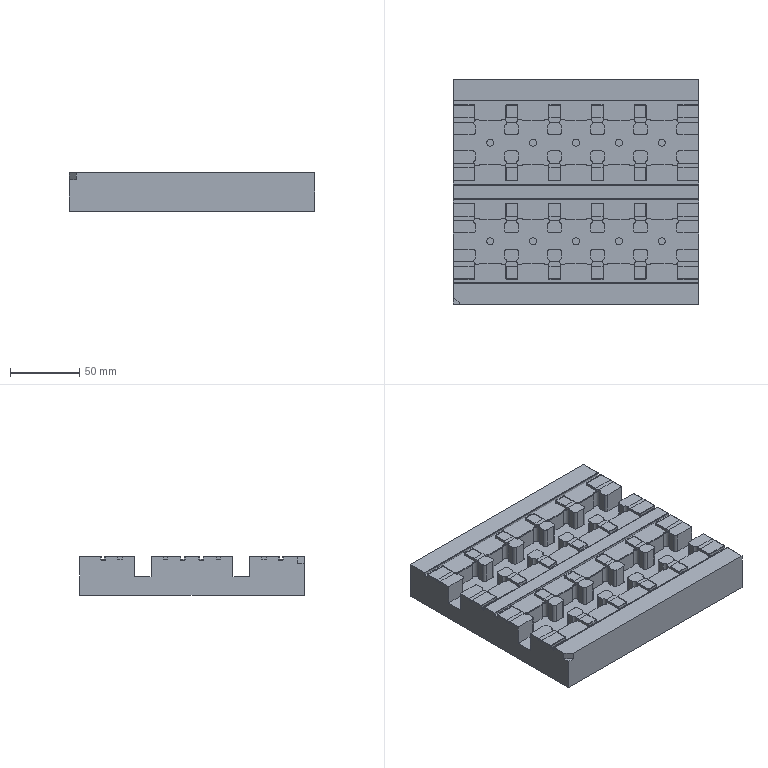NC program | NX | posted by the shop | part box 177 x 162 x 28 mm
Whole program:
%
O0001
(Machine time: 41.63 MIN)
(===Total Tool:4===)
(T2=D17R0.8FlyCutter D=17.  R=0.8  D-  H02 Z=1.    )
(T10=D10    D=10.  R=0.   D10 H10 Z=1.5   )
(T11=D10-J  D=10.  R=0.   D-  H11 Z=1.5   )
(T1=D6ChamferMill   D=6.   R=0.   D-  H01 Z=28.5  )
G80 G90 G17 G49 G40
G91 G28 Z0
M01
N1 T02 M06
(D17R0.8FlyCutter  D=17. R=0.8 H=02 ce=0.20 di=0.10)
(MAX_Z=45. MIN_Z=1. Time=26.17M)
T10
G00 G90 G54 X-109. Y78.971 M03 S2000
G43 H02 Z45.
M08
Z32.3
G01 Z30.3 F3000.
X-97.
X97.
Y68.441
X-97.
Y57.912
X97.
Y47.382
X-97.
Y36.853
X97.
Y26.324
X-97.
Y15.794
X97.
Y5.265
X-97.
Y-5.265
X97.
Y-15.794
X-97.
Y-26.324
X97.
Y-36.853
X-97.
Y-47.382
X97.
Y-57.912
X-97.
Y-68.441
X97.
Y-78.971
X-97.
X-109.
Z32.3
G00 Z33.5
Y78.971
Z32.1
G01 Z30.1
X-97.
X97.
Y68.441
X-97.
Y57.912
X97.
Y47.382
X-97.
Y36.853
X97.
Y26.324
X-97.
Y15.794
X97.
Y5.265
X-97.
Y-5.265
X97.
Y-15.794
X-97.
Y-26.324
X97.
Y-36.853
X-97.
Y-47.382
X97.
Y-57.912
X-97.
Y-68.441
X97.
Y-78.971
X-97.
X-109.
Z32.1
G00 Z45.
G00 G90 X97.2 Y-75.602 M03 S2000
Z45.
Z31.
G01 Y-81.723 Z30.679 F3000.
X96.795 Y-83.722 Z30.572
X95.937 Y-85.572 Z30.465
X94.673 Y-87.173 Z30.359
X93.072 Y-88.437 Z30.252
X91.222 Y-89.295 Z30.145
X89.223 Y-89.7 Z30.038
X88.5 Z30.
X-88.5 Z29.928
G02 X-97.2 Y-81. Z29.922 I0.0 J8.7
G01 Y81. Z29.856
G02 X-88.5 Y89.7 Z29.851 I8.7 J0.0
G01 X88.5 Z29.778
G02 X97.2 Y81. Z29.773 I0.0 J-8.7
G01 Y-81. Z29.707
G02 X88.5 Y-89.7 Z29.701 I-8.7 J0.0
G01 X-88.5 Z29.629
G02 X-97.2 Y-81. Z29.623 I0.0 J8.7
G01 Y81. Z29.557
G02 X-88.5 Y89.7 Z29.552 I8.7 J0.0
G01 X88.5 Z29.479
G02 X97.2 Y81. Z29.474 I0.0 J-8.7
G01 Y-81. Z29.408
G02 X88.5 Y-89.7 Z29.402 I-8.7 J0.0
G01 X-88.5 Z29.33
G02 X-97.2 Y-81. Z29.324 I0.0 J8.7
G01 Y81. Z29.258
G02 X-88.5 Y89.7 Z29.253 I8.7 J0.0
G01 X88.5 Z29.18
G02 X97.2 Y81. Z29.175 I0.0 J-8.7
G01 Y-81. Z29.109
G02 X88.5 Y-89.7 Z29.103 I-8.7 J0.0
G01 X-88.5 Z29.031
G02 X-97.2 Y-81. Z29.025 I0.0 J8.7
G01 Y81. Z28.959
G02 X-88.5 Y89.7 Z28.954 I8.7 J0.0
G01 X88.5 Z28.881
G02 X97.2 Y81. Z28.876 I0.0 J-8.7
G01 Y-81. Z28.81
G02 X88.5 Y-89.7 Z28.804 I-8.7 J0.0
G01 X-88.5 Z28.732
G02 X-97.2 Y-81. Z28.726 I0.0 J8.7
G01 Y81. Z28.66
G02 X-88.5 Y89.7 Z28.655 I8.7 J0.0
G01 X88.5 Z28.582
G02 X97.2 Y81. Z28.577 I0.0 J-8.7
G01 Y-81. Z28.511
G02 X88.5 Y-89.7 Z28.505 I-8.7 J0.0
G01 X-88.5 Z28.433
G02 X-97.2 Y-81. Z28.427 I0.0 J8.7
G01 Y81. Z28.361
G02 X-88.5 Y89.7 Z28.356 I8.7 J0.0
G01 X88.5 Z28.283
G02 X97.2 Y81. Z28.278 I0.0 J-8.7
G01 Y-81. Z28.212
G02 X88.5 Y-89.7 Z28.206 I-8.7 J0.0
G01 X-88.5 Z28.134
G02 X-97.2 Y-81. Z28.128 I0.0 J8.7
G01 Y81. Z28.062
G02 X-88.5 Y89.7 Z28.057 I8.7 J0.0
G01 X88.5 Z27.984
G02 X97.2 Y81. Z27.979 I0.0 J-8.7
G01 Y-81. Z27.913
G02 X88.5 Y-89.7 Z27.907 I-8.7 J0.0
G01 X-88.5 Z27.835
G02 X-97.2 Y-81. Z27.829 I0.0 J8.7
G01 Y81. Z27.763
G02 X-88.5 Y89.7 Z27.758 I8.7 J0.0
G01 X88.5 Z27.686
G02 X97.2 Y81. Z27.68 I0.0 J-8.7
G01 Y-81. Z27.614
G02 X88.5 Y-89.7 Z27.608 I-8.7 J0.0
G01 X-88.5 Z27.536
G02 X-97.2 Y-81. Z27.53 I0.0 J8.7
G01 Y81. Z27.464
G02 X-88.5 Y89.7 Z27.459 I8.7 J0.0
G01 X88.5 Z27.387
G02 X97.2 Y81. Z27.381 I0.0 J-8.7
G01 Y-81. Z27.315
G02 X88.5 Y-89.7 Z27.309 I-8.7 J0.0
G01 X-88.5 Z27.237
G02 X-97.2 Y-81. Z27.231 I0.0 J8.7
G01 Y81. Z27.165
G02 X-88.5 Y89.7 Z27.16 I8.7 J0.0
G01 X88.5 Z27.088
G02 X97.2 Y81. Z27.082 I0.0 J-8.7
G01 Y-81. Z27.016
G02 X88.5 Y-89.7 Z27.01 I-8.7 J0.0
G01 X-88.5 Z26.938
G02 X-97.2 Y-81. Z26.933 I0.0 J8.7
G01 Y81. Z26.866
G02 X-88.5 Y89.7 Z26.861 I8.7 J0.0
G01 X88.5 Z26.789
G02 X97.2 Y81. Z26.783 I0.0 J-8.7
G01 Y-81. Z26.717
G02 X88.5 Y-89.7 Z26.711 I-8.7 J0.0
G01 X-88.5 Z26.639
G02 X-97.2 Y-81. Z26.634 I0.0 J8.7
G01 Y81. Z26.567
G02 X-88.5 Y89.7 Z26.562 I8.7 J0.0
G01 X88.5 Z26.49
G02 X97.2 Y81. Z26.484 I0.0 J-8.7
G01 Y-81. Z26.418
G02 X88.5 Y-89.7 Z26.412 I-8.7 J0.0
G01 X-88.5 Z26.34
G02 X-97.2 Y-81. Z26.335 I0.0 J8.7
G01 Y81. Z26.268
G02 X-88.5 Y89.7 Z26.263 I8.7 J0.0
G01 X88.5 Z26.191
G02 X97.2 Y81. Z26.185 I0.0 J-8.7
G01 Y-81. Z26.119
G02 X88.5 Y-89.7 Z26.113 I-8.7 J0.0
G01 X-88.5 Z26.041
G02 X-97.2 Y-81. Z26.036 I0.0 J8.7
G01 Y81. Z25.969
G02 X-88.5 Y89.7 Z25.964 I8.7 J0.0
G01 X88.5 Z25.892
G02 X97.2 Y81. Z25.886 I0.0 J-8.7
G01 Y-81. Z25.82
G02 X88.5 Y-89.7 Z25.814 I-8.7 J0.0
G01 X-88.5 Z25.742
G02 X-97.2 Y-81. Z25.737 I0.0 J8.7
G01 Y81. Z25.671
G02 X-88.5 Y89.7 Z25.665 I8.7 J0.0
G01 X88.5 Z25.593
G02 X97.2 Y81. Z25.587 I0.0 J-8.7
G01 Y-81. Z25.521
G02 X88.5 Y-89.7 Z25.515 I-8.7 J0.0
G01 X-88.5 Z25.443
G02 X-97.2 Y-81. Z25.438 I0.0 J8.7
G01 Y81. Z25.372
G02 X-88.5 Y89.7 Z25.366 I8.7 J0.0
G01 X88.5 Z25.294
G02 X97.2 Y81. Z25.288 I0.0 J-8.7
G01 Y-81. Z25.222
G02 X88.5 Y-89.7 Z25.216 I-8.7 J0.0
G01 X-88.5 Z25.144
G02 X-97.2 Y-81. Z25.139 I0.0 J8.7
G01 Y81. Z25.073
G02 X-88.5 Y89.7 Z25.067 I8.7 J0.0
G01 X88.5 Z24.995
G02 X97.2 Y81. Z24.989 I0.0 J-8.7
G01 Y-81. Z24.923
G02 X88.5 Y-89.7 Z24.918 I-8.7 J0.0
G01 X-88.5 Z24.845
G02 X-97.2 Y-81. Z24.84 I0.0 J8.7
G01 Y81. Z24.774
G02 X-88.5 Y89.7 Z24.768 I8.7 J0.0
G01 X88.5 Z24.696
G02 X97.2 Y81. Z24.69 I0.0 J-8.7
G01 Y-81. Z24.624
G02 X88.5 Y-89.7 Z24.619 I-8.7 J0.0
G01 X-88.5 Z24.546
G02 X-97.2 Y-81. Z24.541 I0.0 J8.7
G01 Y81. Z24.475
G02 X-88.5 Y89.7 Z24.469 I8.7 J0.0
G01 X88.5 Z24.397
G02 X97.2 Y81. Z24.391 I0.0 J-8.7
G01 Y-81. Z24.325
G02 X88.5 Y-89.7 Z24.32 I-8.7 J0.0
G01 X-88.5 Z24.247
G02 X-97.2 Y-81. Z24.242 I0.0 J8.7
G01 Y81. Z24.176
G02 X-88.5 Y89.7 Z24.17 I8.7 J0.0
G01 X88.5 Z24.098
G02 X97.2 Y81. Z24.092 I0.0 J-8.7
G01 Y-81. Z24.026
G02 X88.5 Y-89.7 Z24.021 I-8.7 J0.0
G01 X-88.5 Z23.948
G02 X-97.2 Y-81. Z23.943 I0.0 J8.7
G01 Y81. Z23.877
G02 X-88.5 Y89.7 Z23.871 I8.7 J0.0
G01 X88.5 Z23.799
G02 X97.2 Y81. Z23.793 I0.0 J-8.7
G01 Y-81. Z23.727
G02 X88.5 Y-89.7 Z23.722 I-8.7 J0.0
G01 X-88.5 Z23.649
G02 X-97.2 Y-81. Z23.644 I0.0 J8.7
G01 Y81. Z23.578
G02 X-88.5 Y89.7 Z23.572 I8.7 J0.0
G01 X88.5 Z23.5
G02 X97.2 Y81. Z23.494 I0.0 J-8.7
G01 Y-81. Z23.428
G02 X88.5 Y-89.7 Z23.423 I-8.7 J0.0
G01 X-88.5 Z23.35
G02 X-97.2 Y-81. Z23.345 I0.0 J8.7
G01 Y81. Z23.279
G02 X-88.5 Y89.7 Z23.273 I8.7 J0.0
G01 X88.5 Z23.201
G02 X97.2 Y81. Z23.195 I0.0 J-8.7
G01 Y-81. Z23.129
G02 X88.5 Y-89.7 Z23.124 I-8.7 J0.0
G01 X-88.5 Z23.051
G02 X-97.2 Y-81. Z23.046 I0.0 J8.7
G01 Y81. Z22.98
G02 X-88.5 Y89.7 Z22.974 I8.7 J0.0
G01 X88.5 Z22.902
G02 X97.2 Y81. Z22.896 I0.0 J-8.7
G01 Y-81. Z22.83
G02 X88.5 Y-89.7 Z22.825 I-8.7 J0.0
G01 X-88.5 Z22.753
G02 X-97.2 Y-81. Z22.747 I0.0 J8.7
G01 Y81. Z22.681
G02 X-88.5 Y89.7 Z22.675 I8.7 J0.0
G01 X88.5 Z22.603
G02 X97.2 Y81. Z22.597 I0.0 J-8.7
G01 Y-81. Z22.531
G02 X88.5 Y-89.7 Z22.526 I-8.7 J0.0
G01 X-88.5 Z22.454
G02 X-97.2 Y-81. Z22.448 I0.0 J8.7
G01 Y81. Z22.382
G02 X-88.5 Y89.7 Z22.376 I8.7 J0.0
G01 X88.5 Z22.304
G02 X97.2 Y81. Z22.298 I0.0 J-8.7
G01 Y-81. Z22.232
G02 X88.5 Y-89.7 Z22.227 I-8.7 J0.0
G01 X-88.5 Z22.155
G02 X-97.2 Y-81. Z22.149 I0.0 J8.7
G01 Y81. Z22.083
G02 X-88.5 Y89.7 Z22.077 I8.7 J0.0
G01 X88.5 Z22.005
G02 X97.2 Y81. Z22. I0.0 J-8.7
G01 Y-81. Z21.933
G02 X88.5 Y-89.7 Z21.928 I-8.7 J0.0
G01 X-88.5 Z21.856
G02 X-97.2 Y-81. Z21.85 I0.0 J8.7
G01 Y81. Z21.784
G02 X-88.5 Y89.7 Z21.778 I8.7 J0.0
G01 X88.5 Z21.706
G02 X97.2 Y81. Z21.701 I0.0 J-8.7
G01 Y-81. Z21.634
G02 X88.5 Y-89.7 Z21.629 I-8.7 J0.0
G01 X-88.5 Z21.557
G02 X-97.2 Y-81. Z21.551 I0.0 J8.7
G01 Y81. Z21.485
G02 X-88.5 Y89.7 Z21.479 I8.7 J0.0
G01 X88.5 Z21.407
G02 X97.2 Y81. Z21.402 I0.0 J-8.7
G01 Y-81. Z21.335
G02 X88.5 Y-89.7 Z21.33 I-8.7 J0.0
G01 X-88.5 Z21.258
G02 X-97.2 Y-81. Z21.252 I0.0 J8.7
G01 Y81. Z21.186
G02 X-88.5 Y89.7 Z21.18 I8.7 J0.0
G01 X88.5 Z21.108
G02 X97.2 Y81. Z21.103 I0.0 J-8.7
G01 Y-81. Z21.037
G02 X88.5 Y-89.7 Z21.031 I-8.7 J0.0
G01 X-88.5 Z20.959
G02 X-97.2 Y-81. Z20.953 I0.0 J8.7
G01 Y81. Z20.887
G02 X-88.5 Y89.7 Z20.881 I8.7 J0.0
G01 X88.5 Z20.809
G02 X97.2 Y81. Z20.804 I0.0 J-8.7
G01 Y-81. Z20.738
G02 X88.5 Y-89.7 Z20.732 I-8.7 J0.0
G01 X-88.5 Z20.66
G02 X-97.2 Y-81. Z20.654 I0.0 J8.7
G01 Y81. Z20.588
G02 X-88.5 Y89.7 Z20.582 I8.7 J0.0
G01 X88.5 Z20.51
G02 X97.2 Y81. Z20.505 I0.0 J-8.7
G01 Y-81. Z20.439
G02 X88.5 Y-89.7 Z20.433 I-8.7 J0.0
G01 X-88.5 Z20.361
G02 X-97.2 Y-81. Z20.355 I0.0 J8.7
G01 Y81. Z20.289
G02 X-88.5 Y89.7 Z20.284 I8.7 J0.0
G01 X88.5 Z20.211
G02 X97.2 Y81. Z20.206 I0.0 J-8.7
G01 Y-81. Z20.14
G02 X88.5 Y-89.7 Z20.134 I-8.7 J0.0
G01 X-88.5 Z20.062
G02 X-97.2 Y-81. Z20.056 I0.0 J8.7
G01 Y81. Z19.99
G02 X-88.5 Y89.7 Z19.985 I8.7 J0.0
G01 X88.5 Z19.912
G02 X97.2 Y81. Z19.907 I0.0 J-8.7
G01 Y-81. Z19.841
G02 X88.5 Y-89.7 Z19.835 I-8.7 J0.0
G01 X-88.5 Z19.763
G02 X-97.2 Y-81. Z19.757 I0.0 J8.7
G01 Y81. Z19.691
G02 X-88.5 Y89.7 Z19.686 I8.7 J0.0
G01 X88.5 Z19.613
G02 X97.2 Y81. Z19.608 I0.0 J-8.7
G01 Y-81. Z19.542
G02 X88.5 Y-89.7 Z19.536 I-8.7 J0.0
G01 X-88.5 Z19.464
G02 X-97.2 Y-81. Z19.458 I0.0 J8.7
G01 Y81. Z19.392
G02 X-88.5 Y89.7 Z19.387 I8.7 J0.0
G01 X88.5 Z19.314
G02 X97.2 Y81. Z19.309 I0.0 J-8.7
G01 Y-81. Z19.243
G02 X88.5 Y-89.7 Z19.237 I-8.7 J0.0
G01 X-88.5 Z19.165
G02 X-97.2 Y-81. Z19.159 I0.0 J8.7
G01 Y81. Z19.093
G02 X-88.5 Y89.7 Z19.088 I8.7 J0.0
G01 X88.5 Z19.015
G02 X97.2 Y81. Z19.01 I0.0 J-8.7
G01 Y-81. Z18.944
G02 X88.5 Y-89.7 Z18.938 I-8.7 J0.0
G01 X-88.5 Z18.866
G02 X-97.2 Y-81. Z18.86 I0.0 J8.7
G01 Y81. Z18.794
G02 X-88.5 Y89.7 Z18.789 I8.7 J0.0
G01 X88.5 Z18.716
G02 X97.2 Y81. Z18.711 I0.0 J-8.7
G01 Y-81. Z18.645
G02 X88.5 Y-89.7 Z18.639 I-8.7 J0.0
G01 X-88.5 Z18.567
G02 X-97.2 Y-81. Z18.561 I0.0 J8.7
G01 Y81. Z18.495
G02 X-88.5 Y89.7 Z18.49 I8.7 J0.0
G01 X88.5 Z18.417
G02 X97.2 Y81. Z18.412 I0.0 J-8.7
G01 Y-81. Z18.346
G02 X88.5 Y-89.7 Z18.34 I-8.7 J0.0
G01 X-88.5 Z18.268
G02 X-97.2 Y-81. Z18.262 I0.0 J8.7
G01 Y81. Z18.196
G02 X-88.5 Y89.7 Z18.191 I8.7 J0.0
G01 X88.5 Z18.118
G02 X97.2 Y81. Z18.113 I0.0 J-8.7
G01 Y-81. Z18.047
G02 X88.5 Y-89.7 Z18.041 I-8.7 J0.0
G01 X-88.5 Z17.969
G02 X-97.2 Y-81. Z17.963 I0.0 J8.7
G01 Y81. Z17.897
G02 X-88.5 Y89.7 Z17.892 I8.7 J0.0
G01 X88.5 Z17.82
G02 X97.2 Y81. Z17.814 I0.0 J-8.7
G01 Y-81. Z17.748
G02 X88.5 Y-89.7 Z17.742 I-8.7 J0.0
G01 X-88.5 Z17.67
G02 X-97.2 Y-81. Z17.664 I0.0 J8.7
G01 Y81. Z17.598
G02 X-88.5 Y89.7 Z17.593 I8.7 J0.0
G01 X88.5 Z17.521
G02 X97.2 Y81. Z17.515 I0.0 J-8.7
G01 Y-81. Z17.449
G02 X88.5 Y-89.7 Z17.443 I-8.7 J0.0
G01 X-88.5 Z17.371
G02 X-97.2 Y-81. Z17.365 I0.0 J8.7
G01 Y81. Z17.299
G02 X-88.5 Y89.7 Z17.294 I8.7 J0.0
G01 X88.5 Z17.222
G02 X97.2 Y81. Z17.216 I0.0 J-8.7
G01 Y-81. Z17.15
G02 X88.5 Y-89.7 Z17.144 I-8.7 J0.0
G01 X-88.5 Z17.072
G02 X-97.2 Y-81. Z17.067 I0.0 J8.7
G01 Y81. Z17.
G02 X-88.5 Y89.7 Z16.995 I8.7 J0.0
G01 X88.5 Z16.923
G02 X97.2 Y81. Z16.917 I0.0 J-8.7
G01 Y-81. Z16.851
G02 X88.5 Y-89.7 Z16.845 I-8.7 J0.0
G01 X-88.5 Z16.773
G02 X-97.2 Y-81. Z16.768 I0.0 J8.7
G01 Y81. Z16.701
G02 X-88.5 Y89.7 Z16.696 I8.7 J0.0
G01 X88.5 Z16.624
G02 X97.2 Y81. Z16.618 I0.0 J-8.7
G01 Y-81. Z16.552
G02 X88.5 Y-89.7 Z16.546 I-8.7 J0.0
G01 X-88.5 Z16.474
G02 X-97.2 Y-81. Z16.469 I0.0 J8.7
G01 Y81. Z16.402
G02 X-88.5 Y89.7 Z16.397 I8.7 J0.0
G01 X88.5 Z16.325
G02 X97.2 Y81. Z16.319 I0.0 J-8.7
G01 Y-81. Z16.253
G02 X88.5 Y-89.7 Z16.247 I-8.7 J0.0
G01 X-88.5 Z16.175
G02 X-97.2 Y-81. Z16.17 I0.0 J8.7
G01 Y81. Z16.104
G02 X-88.5 Y89.7 Z16.098 I8.7 J0.0
G01 X88.5 Z16.026
G02 X97.2 Y81. Z16.02 I0.0 J-8.7
G01 Y-81. Z15.954
G02 X88.5 Y-89.7 Z15.948 I-8.7 J0.0
G01 X-88.5 Z15.876
G02 X-97.2 Y-81. Z15.871 I0.0 J8.7
G01 Y81. Z15.805
G02 X-88.5 Y89.7 Z15.799 I8.7 J0.0
G01 X88.5 Z15.727
G02 X97.2 Y81. Z15.721 I0.0 J-8.7
G01 Y-81. Z15.655
G02 X88.5 Y-89.7 Z15.649 I-8.7 J0.0
G01 X-88.5 Z15.577
G02 X-97.2 Y-81. Z15.572 I0.0 J8.7
G01 Y81. Z15.506
G02 X-88.5 Y89.7 Z15.5 I8.7 J0.0
G01 X88.5 Z15.428
G02 X97.2 Y81. Z15.422 I0.0 J-8.7
G01 Y-81. Z15.356
G02 X88.5 Y-89.7 Z15.351 I-8.7 J0.0
G01 X-88.5 Z15.278
G02 X-97.2 Y-81. Z15.273 I0.0 J8.7
G01 Y81. Z15.207
G02 X-88.5 Y89.7 Z15.201 I8.7 J0.0
G01 X88.5 Z15.129
G02 X97.2 Y81. Z15.123 I0.0 J-8.7
G01 Y-81. Z15.057
G02 X88.5 Y-89.7 Z15.052 I-8.7 J0.0
G01 X-88.5 Z14.979
G02 X-97.2 Y-81. Z14.974 I0.0 J8.7
G01 Y81. Z14.908
G02 X-88.5 Y89.7 Z14.902 I8.7 J0.0
G01 X88.5 Z14.83
G02 X97.2 Y81. Z14.824 I0.0 J-8.7
G01 Y-81. Z14.758
G02 X88.5 Y-89.7 Z14.753 I-8.7 J0.0
G01 X-88.5 Z14.68
G02 X-97.2 Y-81. Z14.675 I0.0 J8.7
G01 Y81. Z14.609
G02 X-88.5 Y89.7 Z14.603 I8.7 J0.0
G01 X88.5 Z14.531
G02 X97.2 Y81. Z14.525 I0.0 J-8.7
G01 Y-81. Z14.459
G02 X88.5 Y-89.7 Z14.454 I-8.7 J0.0
G01 X-88.5 Z14.381
G02 X-97.2 Y-81. Z14.376 I0.0 J8.7
G01 Y81. Z14.31
G02 X-88.5 Y89.7 Z14.304 I8.7 J0.0
G01 X88.5 Z14.232
G02 X97.2 Y81. Z14.226 I0.0 J-8.7
G01 Y-81. Z14.16
G02 X88.5 Y-89.7 Z14.155 I-8.7 J0.0
G01 X-88.5 Z14.082
G02 X-97.2 Y-81. Z14.077 I0.0 J8.7
G01 Y81. Z14.011
G02 X-88.5 Y89.7 Z14.005 I8.7 J0.0
G01 X88.5 Z13.933
G02 X97.2 Y81. Z13.927 I0.0 J-8.7
G01 Y-81. Z13.861
G02 X88.5 Y-89.7 Z13.856 I-8.7 J0.0
G01 X-88.5 Z13.783
G02 X-97.2 Y-81. Z13.778 I0.0 J8.7
G01 Y81. Z13.712
G02 X-88.5 Y89.7 Z13.706 I8.7 J0.0
G01 X88.5 Z13.634
G02 X97.2 Y81. Z13.628 I0.0 J-8.7
G01 Y-81. Z13.562
G02 X88.5 Y-89.7 Z13.557 I-8.7 J0.0
G01 X-88.5 Z13.484
G02 X-97.2 Y-81. Z13.479 I0.0 J8.7
G01 Y81. Z13.413
G02 X-88.5 Y89.7 Z13.407 I8.7 J0.0
G01 X88.5 Z13.335
G02 X97.2 Y81. Z13.329 I0.0 J-8.7
G01 Y-81. Z13.263
G02 X88.5 Y-89.7 Z13.258 I-8.7 J0.0
G01 X-88.5 Z13.186
G02 X-97.2 Y-81. Z13.18 I0.0 J8.7
G01 Y81. Z13.114
G02 X-88.5 Y89.7 Z13.108 I8.7 J0.0
G01 X88.5 Z13.036
G02 X97.2 Y81. Z13.03 I0.0 J-8.7
G01 Y-81. Z12.964
G02 X88.5 Y-89.7 Z12.959 I-8.7 J0.0
G01 X-88.5 Z12.887
G02 X-97.2 Y-81. Z12.881 I0.0 J8.7
G01 Y81. Z12.815
G02 X-88.5 Y89.7 Z12.809 I8.7 J0.0
G01 X88.5 Z12.737
G02 X97.2 Y81. Z12.731 I0.0 J-8.7
G01 Y-81. Z12.665
G02 X88.5 Y-89.7 Z12.66 I-8.7 J0.0
G01 X-88.5 Z12.588
G02 X-97.2 Y-81. Z12.582 I0.0 J8.7
G01 Y81. Z12.516
G02 X-88.5 Y89.7 Z12.51 I8.7 J0.0
G01 X88.5 Z12.438
G02 X97.2 Y81. Z12.433 I0.0 J-8.7
G01 Y-81. Z12.366
G02 X88.5 Y-89.7 Z12.361 I-8.7 J0.0
G01 X-88.5 Z12.289
G02 X-97.2 Y-81. Z12.283 I0.0 J8.7
G01 Y81. Z12.217
G02 X-88.5 Y89.7 Z12.211 I8.7 J0.0
G01 X88.5 Z12.139
G02 X97.2 Y81. Z12.134 I0.0 J-8.7
G01 Y-81. Z12.067
G02 X88.5 Y-89.7 Z12.062 I-8.7 J0.0
G01 X-88.5 Z11.99
G02 X-97.2 Y-81. Z11.984 I0.0 J8.7
G01 Y81. Z11.918
G02 X-88.5 Y89.7 Z11.912 I8.7 J0.0
G01 X88.5 Z11.84
G02 X97.2 Y81. Z11.835 I0.0 J-8.7
G01 Y-81. Z11.768
G02 X88.5 Y-89.7 Z11.763 I-8.7 J0.0
G01 X-88.5 Z11.691
G02 X-97.2 Y-81. Z11.685 I0.0 J8.7
G01 Y81. Z11.619
G02 X-88.5 Y89.7 Z11.613 I8.7 J0.0
G01 X88.5 Z11.541
G02 X97.2 Y81. Z11.536 I0.0 J-8.7
G01 Y-81. Z11.469
G02 X88.5 Y-89.7 Z11.464 I-8.7 J0.0
G01 X-88.5 Z11.392
G02 X-97.2 Y-81. Z11.386 I0.0 J8.7
G01 Y81. Z11.32
G02 X-88.5 Y89.7 Z11.314 I8.7 J0.0
G01 X88.5 Z11.242
G02 X97.2 Y81. Z11.237 I0.0 J-8.7
G01 Y-81. Z11.171
G02 X88.5 Y-89.7 Z11.165 I-8.7 J0.0
G01 X-88.5 Z11.093
G02 X-97.2 Y-81. Z11.087 I0.0 J8.7
G01 Y81. Z11.021
G02 X-88.5 Y89.7 Z11.015 I8.7 J0.0
G01 X88.5 Z10.943
G02 X97.2 Y81. Z10.938 I0.0 J-8.7
G01 Y-81. Z10.872
G02 X88.5 Y-89.7 Z10.866 I-8.7 J0.0
G01 X-88.5 Z10.794
G02 X-97.2 Y-81. Z10.788 I0.0 J8.7
G01 Y81. Z10.722
G02 X-88.5 Y89.7 Z10.716 I8.7 J0.0
G01 X88.5 Z10.644
G02 X97.2 Y81. Z10.639 I0.0 J-8.7
G01 Y-81. Z10.573
G02 X88.5 Y-89.7 Z10.567 I-8.7 J0.0
G01 X-88.5 Z10.495
G02 X-97.2 Y-81. Z10.489 I0.0 J8.7
G01 Y81. Z10.423
G02 X-88.5 Y89.7 Z10.418 I8.7 J0.0
G01 X88.5 Z10.345
G02 X97.2 Y81. Z10.34 I0.0 J-8.7
G01 Y-81. Z10.274
G02 X88.5 Y-89.7 Z10.268 I-8.7 J0.0
G01 X-88.5 Z10.196
G02 X-97.2 Y-81. Z10.19 I0.0 J8.7
G01 Y81. Z10.124
G02 X-88.5 Y89.7 Z10.119 I8.7 J0.0
G01 X88.5 Z10.046
G02 X97.2 Y81. Z10.041 I0.0 J-8.7
G01 Y-81. Z9.975
G02 X88.5 Y-89.7 Z9.969 I-8.7 J0.0
G01 X-88.5 Z9.897
G02 X-97.2 Y-81. Z9.891 I0.0 J8.7
G01 Y81. Z9.825
G02 X-88.5 Y89.7 Z9.82 I8.7 J0.0
G01 X88.5 Z9.747
G02 X97.2 Y81. Z9.742 I0.0 J-8.7
G01 Y-81. Z9.676
G02 X88.5 Y-89.7 Z9.67 I-8.7 J0.0
G01 X-88.5 Z9.598
G02 X-97.2 Y-81. Z9.592 I0.0 J8.7
G01 Y81. Z9.526
G02 X-88.5 Y89.7 Z9.521 I8.7 J0.0
G01 X88.5 Z9.448
G02 X97.2 Y81. Z9.443 I0.0 J-8.7
G01 Y-81. Z9.377
G02 X88.5 Y-89.7 Z9.371 I-8.7 J0.0
G01 X-88.5 Z9.299
G02 X-97.2 Y-81. Z9.293 I0.0 J8.7
G01 Y81. Z9.227
G02 X-88.5 Y89.7 Z9.222 I8.7 J0.0
G01 X88.5 Z9.149
G02 X97.2 Y81. Z9.144 I0.0 J-8.7
G01 Y-81. Z9.078
G02 X88.5 Y-89.7 Z9.072 I-8.7 J0.0
G01 X-88.5 Z9.
G02 X-97.2 Y-81. Z8.994 I0.0 J8.7
G01 Y81. Z8.928
G02 X-88.5 Y89.7 Z8.923 I8.7 J0.0
G01 X88.5 Z8.85
G02 X97.2 Y81. Z8.845 I0.0 J-8.7
G01 Y-81. Z8.779
G02 X88.5 Y-89.7 Z8.773 I-8.7 J0.0
G01 X-88.5 Z8.701
G02 X-97.2 Y-81. Z8.695 I0.0 J8.7
G01 Y81. Z8.629
G02 X-88.5 Y89.7 Z8.624 I8.7 J0.0
G01 X88.5 Z8.551
G02 X97.2 Y81. Z8.546 I0.0 J-8.7
G01 Y-81. Z8.48
G02 X88.5 Y-89.7 Z8.474 I-8.7 J0.0
G01 X-88.5 Z8.402
G02 X-97.2 Y-81. Z8.396 I0.0 J8.7
G01 Y81. Z8.33
G02 X-88.5 Y89.7 Z8.325 I8.7 J0.0
G01 X88.5 Z8.253
G02 X97.2 Y81. Z8.247 I0.0 J-8.7
G01 Y-81. Z8.181
G02 X88.5 Y-89.7 Z8.175 I-8.7 J0.0
G01 X-88.5 Z8.103
G02 X-97.2 Y-81. Z8.097 I0.0 J8.7
G01 Y81. Z8.031
G02 X-88.5 Y89.7 Z8.026 I8.7 J0.0
G01 X88.5 Z7.954
G02 X97.2 Y81. Z7.948 I0.0 J-8.7
G01 Y-81. Z7.882
G02 X88.5 Y-89.7 Z7.876 I-8.7 J0.0
G01 X-88.5 Z7.804
G02 X-97.2 Y-81. Z7.798 I0.0 J8.7
G01 Y81. Z7.732
G02 X-88.5 Y89.7 Z7.727 I8.7 J0.0
G01 X88.5 Z7.655
G02 X97.2 Y81. Z7.649 I0.0 J-8.7
G01 Y-81. Z7.583
G02 X88.5 Y-89.7 Z7.577 I-8.7 J0.0
G01 X-88.5 Z7.505
G02 X-97.2 Y-81. Z7.5 I0.0 J8.7
G01 Y81. Z7.433
G02 X-88.5 Y89.7 Z7.428 I8.7 J0.0
G01 X88.5 Z7.356
G02 X97.2 Y81. Z7.35 I0.0 J-8.7
G01 Y-81. Z7.284
G02 X88.5 Y-89.7 Z7.278 I-8.7 J0.0
G01 X-88.5 Z7.206
G02 X-97.2 Y-81. Z7.201 I0.0 J8.7
G01 Y81. Z7.134
G02 X-88.5 Y89.7 Z7.129 I8.7 J0.0
G01 X88.5 Z7.057
G02 X97.2 Y81. Z7.051 I0.0 J-8.7
G01 Y-81. Z6.985
G02 X88.5 Y-89.7 Z6.979 I-8.7 J0.0
G01 X-88.5 Z6.907
G02 X-97.2 Y-81. Z6.902 I0.0 J8.7
G01 Y81. Z6.835
G02 X-88.5 Y89.7 Z6.83 I8.7 J0.0
G01 X88.5 Z6.758
G02 X97.2 Y81. Z6.752 I0.0 J-8.7
G01 Y-81. Z6.686
G02 X88.5 Y-89.7 Z6.68 I-8.7 J0.0
G01 X-88.5 Z6.608
G02 X-97.2 Y-81. Z6.603 I0.0 J8.7
G01 Y81. Z6.537
G02 X-88.5 Y89.7 Z6.531 I8.7 J0.0
G01 X88.5 Z6.459
G02 X97.2 Y81. Z6.453 I0.0 J-8.7
G01 Y-81. Z6.387
G02 X88.5 Y-89.7 Z6.381 I-8.7 J0.0
G01 X-88.5 Z6.309
G02 X-97.2 Y-81. Z6.304 I0.0 J8.7
G01 Y81. Z6.238
G02 X-88.5 Y89.7 Z6.232 I8.7 J0.0
G01 X88.5 Z6.16
G02 X97.2 Y81. Z6.154 I0.0 J-8.7
G01 Y-81. Z6.088
G02 X88.5 Y-89.7 Z6.082 I-8.7 J0.0
G01 X-88.5 Z6.01
G02 X-97.2 Y-81. Z6.005 I0.0 J8.7
G01 Y81. Z5.939
G02 X-88.5 Y89.7 Z5.933 I8.7 J0.0
G01 X88.5 Z5.861
G02 X97.2 Y81. Z5.855 I0.0 J-8.7
G01 Y-81. Z5.789
G02 X88.5 Y-89.7 Z5.784 I-8.7 J0.0
G01 X-88.5 Z5.711
G02 X-97.2 Y-81. Z5.706 I0.0 J8.7
G01 Y81. Z5.64
G02 X-88.5 Y89.7 Z5.634 I8.7 J0.0
G01 X88.5 Z5.562
G02 X97.2 Y81. Z5.556 I0.0 J-8.7
G01 Y-81. Z5.49
G02 X88.5 Y-89.7 Z5.485 I-8.7 J0.0
G01 X-88.5 Z5.412
G02 X-97.2 Y-81. Z5.407 I0.0 J8.7
G01 Y81. Z5.341
G02 X-88.5 Y89.7 Z5.335 I8.7 J0.0
G01 X88.5 Z5.263
G02 X97.2 Y81. Z5.257 I0.0 J-8.7
G01 Y-81. Z5.191
G02 X88.5 Y-89.7 Z5.186 I-8.7 J0.0
G01 X-88.5 Z5.113
G02 X-97.2 Y-81. Z5.108 I0.0 J8.7
G01 Y81. Z5.042
G02 X-88.5 Y89.7 Z5.036 I8.7 J0.0
G01 X88.5 Z4.964
G02 X97.2 Y81. Z4.958 I0.0 J-8.7
G01 Y-81. Z4.892
G02 X88.5 Y-89.7 Z4.887 I-8.7 J0.0
G01 X-88.5 Z4.814
G02 X-97.2 Y-81. Z4.809 I0.0 J8.7
G01 Y81. Z4.743
G02 X-88.5 Y89.7 Z4.737 I8.7 J0.0
G01 X88.5 Z4.665
G02 X97.2 Y81. Z4.659 I0.0 J-8.7
G01 Y-81. Z4.593
G02 X88.5 Y-89.7 Z4.588 I-8.7 J0.0
G01 X-88.5 Z4.515
G02 X-97.2 Y-81. Z4.51 I0.0 J8.7
G01 Y81. Z4.444
G02 X-88.5 Y89.7 Z4.438 I8.7 J0.0
G01 X88.5 Z4.366
G02 X97.2 Y81. Z4.36 I0.0 J-8.7
G01 Y-81. Z4.294
G02 X88.5 Y-89.7 Z4.289 I-8.7 J0.0
G01 X-88.5 Z4.216
G02 X-97.2 Y-81. Z4.211 I0.0 J8.7
G01 Y81. Z4.145
G02 X-88.5 Y89.7 Z4.139 I8.7 J0.0
G01 X88.5 Z4.067
G02 X97.2 Y81. Z4.061 I0.0 J-8.7
G01 Y-81. Z3.995
G02 X88.5 Y-89.7 Z3.99 I-8.7 J0.0
G01 X-88.5 Z3.917
G02 X-97.2 Y-81. Z3.912 I0.0 J8.7
G01 Y81. Z3.846
G02 X-88.5 Y89.7 Z3.84 I8.7 J0.0
G01 X88.5 Z3.768
G02 X97.2 Y81. Z3.762 I0.0 J-8.7
G01 Y-81. Z3.696
G02 X88.5 Y-89.7 Z3.691 I-8.7 J0.0
G01 X-88.5 Z3.618
G02 X-97.2 Y-81. Z3.613 I0.0 J8.7
G01 Y81. Z3.547
G02 X-88.5 Y89.7 Z3.541 I8.7 J0.0
G01 X88.5 Z3.469
G02 X97.2 Y81. Z3.463 I0.0 J-8.7
G01 Y-81. Z3.397
G02 X88.5 Y-89.7 Z3.392 I-8.7 J0.0
G01 X-88.5 Z3.32
G02 X-97.2 Y-81. Z3.314 I0.0 J8.7
G01 Y81. Z3.248
G02 X-88.5 Y89.7 Z3.242 I8.7 J0.0
G01 X88.5 Z3.17
G02 X97.2 Y81. Z3.164 I0.0 J-8.7
G01 Y-81. Z3.098
G02 X88.5 Y-89.7 Z3.093 I-8.7 J0.0
G01 X-88.5 Z3.021
G02 X-97.2 Y-81. Z3.015 I0.0 J8.7
G01 Y81. Z2.949
G02 X-88.5 Y89.7 Z2.943 I8.7 J0.0
G01 X88.5 Z2.871
G02 X97.2 Y81. Z2.865 I0.0 J-8.7
G01 Y-81. Z2.799
G02 X88.5 Y-89.7 Z2.794 I-8.7 J0.0
G01 X-88.5 Z2.722
G02 X-97.2 Y-81. Z2.716 I0.0 J8.7
G01 Y81. Z2.65
G02 X-88.5 Y89.7 Z2.644 I8.7 J0.0
G01 X88.5 Z2.572
G02 X97.2 Y81. Z2.567 I0.0 J-8.7
G01 Y-81. Z2.5
G02 X88.5 Y-89.7 Z2.495 I-8.7 J0.0
G01 X-88.5 Z2.423
G02 X-97.2 Y-81. Z2.417 I0.0 J8.7
G01 Y81. Z2.351
G02 X-88.5 Y89.7 Z2.345 I8.7 J0.0
G01 X88.5 Z2.273
G02 X97.2 Y81. Z2.268 I0.0 J-8.7
G01 Y-81. Z2.201
G02 X88.5 Y-89.7 Z2.196 I-8.7 J0.0
G01 X-88.5 Z2.124
G02 X-97.2 Y-81. Z2.118 I0.0 J8.7
G01 Y81. Z2.052
G02 X-88.5 Y89.7 Z2.046 I8.7 J0.0
G01 X88.5 Z1.974
G02 X97.2 Y81. Z1.969 I0.0 J-8.7
G01 Y-81. Z1.902
G02 X88.5 Y-89.7 Z1.897 I-8.7 J0.0
G01 X-88.5 Z1.825
G02 X-97.2 Y-81. Z1.819 I0.0 J8.7
G01 Y81. Z1.753
G02 X-88.5 Y89.7 Z1.747 I8.7 J0.0
G01 X88.5 Z1.675
G02 X97.2 Y81. Z1.67 I0.0 J-8.7
G01 Y-81. Z1.604
G02 X88.5 Y-89.7 Z1.598 I-8.7 J0.0
G01 X-88.5 Z1.526
G02 X-97.2 Y-81. Z1.52 I0.0 J8.7
G01 Y81. Z1.454
G02 X-88.5 Y89.7 Z1.448 I8.7 J0.0
G01 X88.5 Z1.376
G02 X97.2 Y81. Z1.371 I0.0 J-8.7
G01 Y-81. Z1.305
G02 X88.5 Y-89.7 Z1.299 I-8.7 J0.0
G01 X-88.5 Z1.227
G02 X-97.2 Y-81. Z1.221 I0.0 J8.7
G01 Y81. Z1.155
G02 X-88.5 Y89.7 Z1.149 I8.7 J0.0
G01 X88.5 Z1.077
G02 X97.2 Y81. Z1.072 I0.0 J-8.7
G01 Y-81. Z1.006
G02 X88.5 Y-89.7 Z1. I-8.7 J0.0
G01 X-88.5
G02 X-97.2 Y-81. I0.0 J8.7
G01 Y81.
G02 X-88.5 Y89.7 I8.7 J0.0
G01 X88.5
G02 X97.2 Y81. I0.0 J-8.7
G01 Y-81.
G02 X88.5 Y-89.7 I-8.7 J0.0
G01 X88.1
Z2.
G00 Z45.
G91 G28 Z0.0
M05
M09
G91 G28 Z0.0
M01
N2 T10 M06
(D10  D=10. R=0. H=10 ce=0.05 di=0.30)
(D.N=10 MAX_Z=45. MIN_Z=1.5 Time=2.87M)
T11
G00 G90 G54 X89.532 Y-86.944 M03 S3000
G43 H10 Z45.
M08
Z25.75
G01 Z25.25 F1500.
G41 D10
X89.327 Y-86.488
G03 X88.5 Y-86.05 I-.827 J-.562
G01 X-88.5
G02 X-93.55 Y-81. I0.0 J5.05
G01 Y81.
G02 X-88.5 Y86.05 I5.05 J0.0
G01 X88.5
G02 X93.55 Y81. I0.0 J-5.05
G01 Y-81.
G02 X88.5 Y-86.05 I-5.05 J0.0
G01 X88.
G03 X87.134 Y-86.55 I0.0 J-1.
G01 G40 X86.963 Y-87.02
Z25.75
G00 Z30.5
X89.532 Y-86.944
Z21.
G01 Z20.5
G41 D10
X89.327 Y-86.488
G03 X88.5 Y-86.05 I-.827 J-.562
G01 X-88.5
G02 X-93.55 Y-81. I0.0 J5.05
G01 Y81.
G02 X-88.5 Y86.05 I5.05 J0.0
G01 X88.5
G02 X93.55 Y81. I0.0 J-5.05
G01 Y-81.
G02 X88.5 Y-86.05 I-5.05 J0.0
G01 X88.
G03 X87.134 Y-86.55 I0.0 J-1.
G01 G40 X86.963 Y-87.02
Z21.
G00 Z25.75
X89.532 Y-86.944
Z16.25
G01 Z15.75
G41 D10
X89.327 Y-86.488
G03 X88.5 Y-86.05 I-.827 J-.562
G01 X-88.5
G02 X-93.55 Y-81. I0.0 J5.05
G01 Y81.
G02 X-88.5 Y86.05 I5.05 J0.0
G01 X88.5
G02 X93.55 Y81. I0.0 J-5.05
G01 Y-81.
G02 X88.5 Y-86.05 I-5.05 J0.0
G01 X88.
G03 X87.134 Y-86.55 I0.0 J-1.
G01 G40 X86.963 Y-87.02
Z16.25
G00 Z21.
X89.532 Y-86.944
Z11.5
G01 Z11.
G41 D10
X89.327 Y-86.488
G03 X88.5 Y-86.05 I-.827 J-.562
G01 X-88.5
G02 X-93.55 Y-81. I0.0 J5.05
G01 Y81.
G02 X-88.5 Y86.05 I5.05 J0.0
G01 X88.5
G02 X93.55 Y81. I0.0 J-5.05
G01 Y-81.
G02 X88.5 Y-86.05 I-5.05 J0.0
G01 X88.
G03 X87.134 Y-86.55 I0.0 J-1.
G01 G40 X86.963 Y-87.02
Z11.5
G00 Z16.25
X89.532 Y-86.944
Z6.75
G01 Z6.25
G41 D10
X89.327 Y-86.488
G03 X88.5 Y-86.05 I-.827 J-.562
G01 X-88.5
G02 X-93.55 Y-81. I0.0 J5.05
G01 Y81.
G02 X-88.5 Y86.05 I5.05 J0.0
G01 X88.5
G02 X93.55 Y81. I0.0 J-5.05
G01 Y-81.
G02 X88.5 Y-86.05 I-5.05 J0.0
G01 X88.
G03 X87.134 Y-86.55 I0.0 J-1.
G01 G40 X86.963 Y-87.02
Z6.75
G00 Z11.5
X89.532 Y-86.944
Z2.
G01 Z1.5
G41 D10
X89.327 Y-86.488
G03 X88.5 Y-86.05 I-.827 J-.562
G01 X-88.5
G02 X-93.55 Y-81. I0.0 J5.05
G01 Y81.
G02 X-88.5 Y86.05 I5.05 J0.0
G01 X88.5
G02 X93.55 Y81. I0.0 J-5.05
G01 Y-81.
G02 X88.5 Y-86.05 I-5.05 J0.0
G01 X88.
G03 X87.134 Y-86.55 I0.0 J-1.
G01 G40 X86.963 Y-87.02
Z2.
G00 Z45.
G91 G28 Z0.0
M05
M09
G91 G28 Z0.0
M01
N3 T11 M06
(D10-J  D=10. R=0. H=11 ce=0.00 di=0.00)
(MAX_Z=45. MIN_Z=30. Time=6.57M)
T01
G00 G90 G54 X-105.5 Y81.086 M03 S3000
G43 H11 Z45.
M08
Z32.
G01 Z30. F1000.
X-93.5
X93.5
Y76.171
X-93.5
Y71.257
X93.5
Y66.343
X-93.5
Y61.429
X93.5
Y56.514
X-93.5
Y51.6
X93.5
Y46.686
X-93.5
Y41.771
X93.5
Y36.857
X-93.5
Y31.943
X93.5
Y27.029
X-93.5
Y22.114
X93.5
Y17.2
X-93.5
Y12.286
X93.5
Y7.371
X-93.5
Y2.457
X93.5
Y-2.457
X-93.5
Y-7.371
X93.5
Y-12.286
X-93.5
Y-17.2
X93.5
Y-22.114
X-93.5
Y-27.029
X93.5
Y-31.943
X-93.5
Y-36.857
X93.5
Y-41.771
X-93.5
Y-46.686
X93.5
Y-51.6
X-93.5
Y-56.514
X93.5
Y-61.429
X-93.5
Y-66.343
X93.5
Y-71.257
X-93.5
Y-76.171
X93.5
Y-81.086
X-93.5
X-105.5
Z32.
G00 Z45.
G91 G28 Z0.0
M05
M09
G91 G28 Z0.0
M01
N4 T01 M06
(D6ChamferMill  D=6. R=0. H=01 ce=0.00 di=0.00)
(MAX_Z=45. MIN_Z=28.5 Time=0.70M)
T11
G00 G90 G54 X.25 Y-83.128 M03 S3000
G43 H01 Z45.
M08
Z32.099
G01 Z28.5 F1000.
G03 X.33 Y-82.828 I-.52 J.3
X.03 Y-82.308 I-.6 J0.0
G01 X0.0 Y-82.3
X-88.5
G02 X-89.8 Y-81. I0.0 J1.3
G01 Y81.
G02 X-88.5 Y82.3 I1.3 J0.0
G01 X88.5
G02 X89.8 Y81. I0.0 J-1.3
G01 Y-81.
G02 X88.5 Y-82.3 I-1.3 J0.0
G01 X0.0
X-.03 Y-82.308
G03 X-.33 Y-82.828 I.3 J-.52
X-.25 Y-83.128 I.6 J0.0
G01 Z32.099
G00 Z45.
G91 G28 Z0.0
M05
M09
G91 G28 Z0.0
M01
N5 T11 M06
(D10-J  D=10. R=0. H=11 ce=0.00 di=0.20)
(D.N=11 MAX_Z=45. MIN_Z=1.5 Time=4.32M)
T02
G00 G90 G54 X-89.513 Y87.126 M03 S3000
G43 H11 Z45.
M08
Z21.
G01 Z20.5 F1000.
G41 D11
X-89.497 Y86.927
G03 X-88.5 Y86.01 I.997 J.083
G01 X88.5
G02 X93.51 Y81. I0.0 J-5.01
G01 Y-81.
G02 X88.5 Y-86.01 I-5.01 J0.0
G01 X-88.5
G02 X-93.51 Y-81. I0.0 J5.01
G01 Y81.
G02 X-88.5 Y86.01 I5.01 J0.0
G01 X-88.
G03 X-87. Y87.01 I0.0 J1.
G01 G40 Y87.21
X-89.512 Y87.126
G41 D11
X-89.497 Y86.927
G03 X-88.5 Y86. I.997 J.073
G01 X88.5
G02 X93.5 Y81. I0.0 J-5.
G01 Y-81.
G02 X88.5 Y-86. I-5. J0.0
G01 X-88.5
G02 X-93.5 Y-81. I0.0 J5.
G01 Y81.
G02 X-88.5 Y86. I5. J0.0
G01 X-88.
G03 X-87. Y87. I0.0 J1.
G01 Y87.01
G40 Y87.21
Z21.
G00 Z45.
X-89.513 Y87.126
Z11.5
G01 Z11.
G41 D11
X-89.497 Y86.927
G03 X-88.5 Y86.01 I.997 J.083
G01 X88.5
G02 X93.51 Y81. I0.0 J-5.01
G01 Y-81.
G02 X88.5 Y-86.01 I-5.01 J0.0
G01 X-88.5
G02 X-93.51 Y-81. I0.0 J5.01
G01 Y81.
G02 X-88.5 Y86.01 I5.01 J0.0
G01 X-88.
G03 X-87. Y87.01 I0.0 J1.
G01 G40 Y87.21
X-89.512 Y87.126
G41 D11
X-89.497 Y86.927
G03 X-88.5 Y86. I.997 J.073
G01 X88.5
G02 X93.5 Y81. I0.0 J-5.
G01 Y-81.
G02 X88.5 Y-86. I-5. J0.0
G01 X-88.5
G02 X-93.5 Y-81. I0.0 J5.
G01 Y81.
G02 X-88.5 Y86. I5. J0.0
G01 X-88.
G03 X-87. Y87. I0.0 J1.
G01 Y87.01
G40 Y87.21
Z11.5
G00 Z45.
X-89.513 Y87.126
Z2.
G01 Z1.5
G41 D11
X-89.497 Y86.927
G03 X-88.5 Y86.01 I.997 J.083
G01 X88.5
G02 X93.51 Y81. I0.0 J-5.01
G01 Y-81.
G02 X88.5 Y-86.01 I-5.01 J0.0
G01 X-88.5
G02 X-93.51 Y-81. I0.0 J5.01
G01 Y81.
G02 X-88.5 Y86.01 I5.01 J0.0
G01 X-88.
G03 X-87. Y87.01 I0.0 J1.
G01 G40 Y87.21
X-89.512 Y87.126
G41 D11
X-89.497 Y86.927
G03 X-88.5 Y86. I.997 J.073
G01 X88.5
G02 X93.5 Y81. I0.0 J-5.
G01 Y-81.
G02 X88.5 Y-86. I-5. J0.0
G01 X-88.5
G02 X-93.5 Y-81. I0.0 J5.
G01 Y81.
G02 X-88.5 Y86. I5. J0.0
G01 X-88.
G03 X-87. Y87. I0.0 J1.
G01 Y87.01
G40 Y87.21
Z2.
G00 Z45.
M05
M09
G91 G28 Z0.0
G91 G28 Y0.0
M30
%